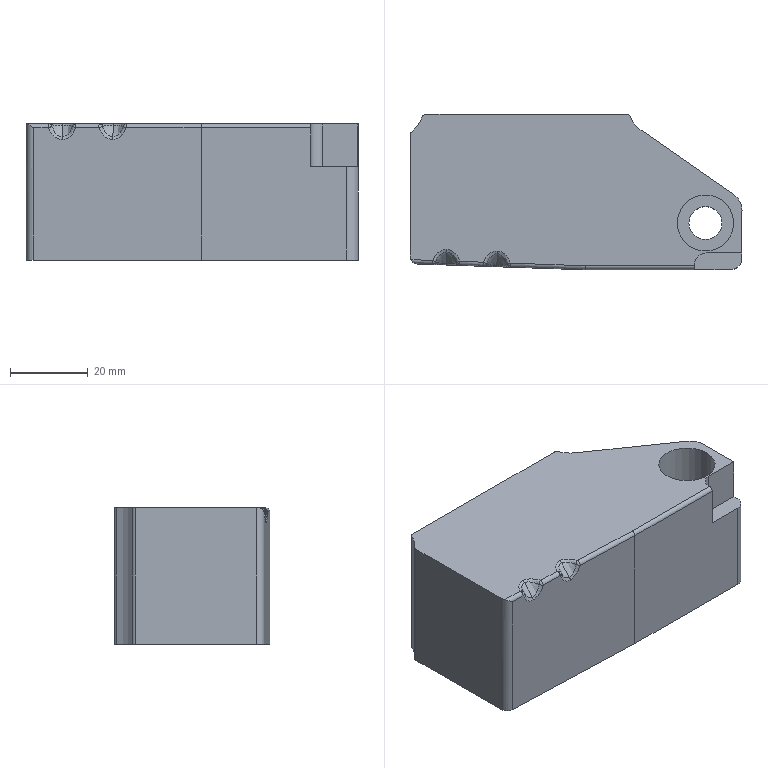Part | NX | features DIE-82 2 | 1 solid | 45 faces | box 85.4 x 40 x 35 mm | volume 101853 mm3 | cylinder 15 | plane 13 | spline 12 | sphere 5 | commonest cylinder face diameters 2 x7 6 x2 4 x1 8.5 x1 10 x1 14.5 x1